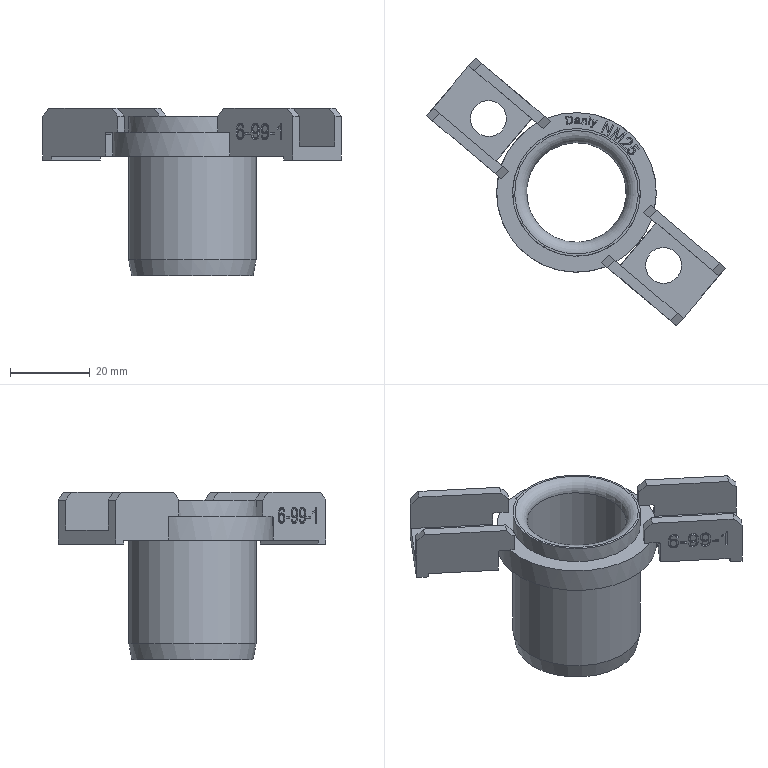Part | STEP file | lll_id4590_x_t | 1 solid | 237 faces | box 74.888 x 67.123 x 42 mm | volume 18803 mm3 | plane 156 | other 69 | cylinder 10 | torus 1 | cone 1 | commonest cylinder face diameters 1 x4 9 x2 32 x2 25 x1 40 x1